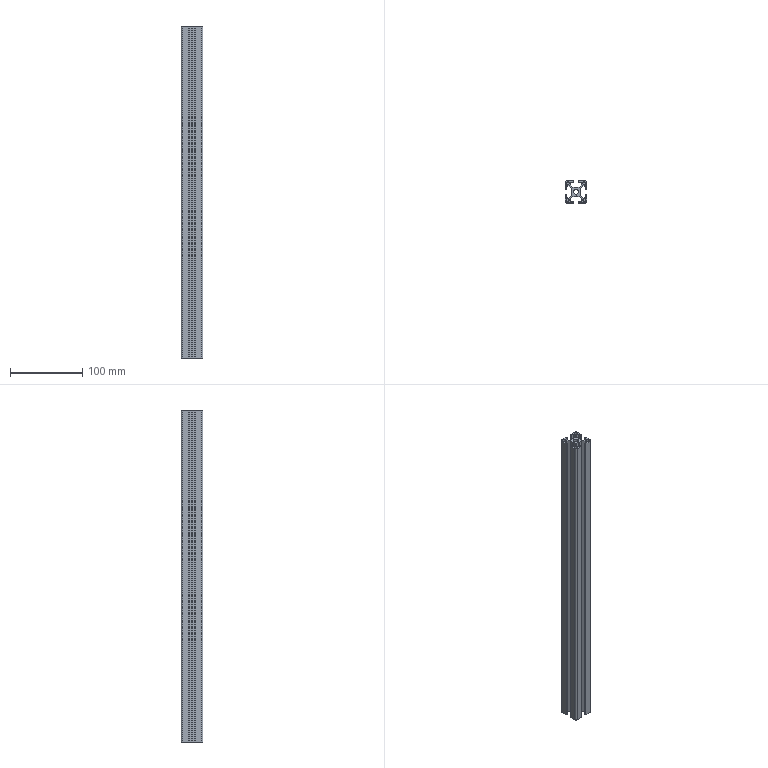Part | STEP file | SQ-8-3030W-460_Default | 1 solid | 84 faces | box 30 x 30 x 460 mm | volume 172560 mm3 | plane 62 | cylinder 22 | commonest cylinder face diameters 0.6 x8 4.2 x8 4 x4 6.8 x2